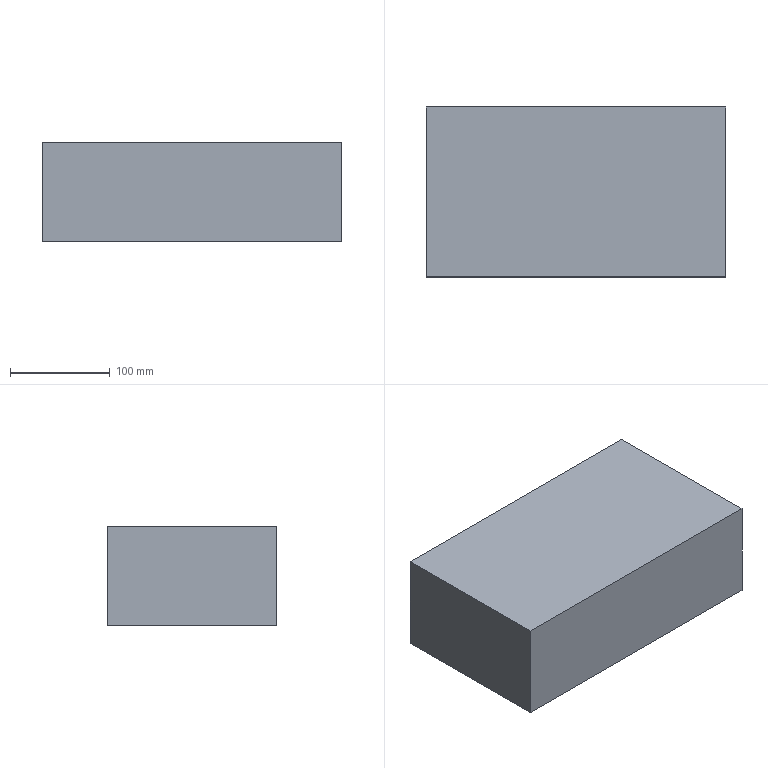Part | SolidWorks | features Extrusion 1 | 1 solid | 6 faces | box 300 x 170 x 100 mm | volume 5100000 mm3 | plane 6
STEP:
#1=CARTESIAN_POINT('',(-150.,85.,50.));
#2=VERTEX_POINT('',#1);
#3=CARTESIAN_POINT('',(-150.,-85.,50.));
#4=VERTEX_POINT('',#3);
#5=CARTESIAN_POINT('',(-150.,85.,50.));
#6=DIRECTION('',(0.,-1.,0.));
#7=VECTOR('',#6,1000.);
#8=LINE('',#5,#7);
#9=EDGE_CURVE('',#2,#4,#8,.T.);
#10=ORIENTED_EDGE('',*,*,#9,.F.);
#11=CARTESIAN_POINT('',(-150.,85.,-50.));
#12=VERTEX_POINT('',#11);
#13=CARTESIAN_POINT('',(-150.,85.,-50.));
#14=DIRECTION('',(0.,0.,1.));
#15=VECTOR('',#14,1000.);
#16=LINE('',#13,#15);
#17=EDGE_CURVE('',#12,#2,#16,.T.);
#18=ORIENTED_EDGE('',*,*,#17,.F.);
#19=CARTESIAN_POINT('',(-150.,-85.,-50.));
#20=VERTEX_POINT('',#19);
#21=CARTESIAN_POINT('',(-150.,85.,-50.));
#22=DIRECTION('',(0.,-1.,0.));
#23=VECTOR('',#22,1000.);
#24=LINE('',#21,#23);
#25=EDGE_CURVE('',#12,#20,#24,.T.);
#26=ORIENTED_EDGE('',*,*,#25,.T.);
#27=CARTESIAN_POINT('',(-150.,-85.,-50.));
#28=DIRECTION('',(0.,0.,1.));
#29=VECTOR('',#28,1000.);
#30=LINE('',#27,#29);
#31=EDGE_CURVE('',#20,#4,#30,.T.);
#32=ORIENTED_EDGE('',*,*,#31,.T.);
#33=EDGE_LOOP('',(#10,#18,#26,#32));
#34=FACE_OUTER_BOUND('',#33,.T.);
#35=CARTESIAN_POINT('',(-150.,85.,-50.));
#36=DIRECTION('',(-1.,0.,0.));
#37=DIRECTION('',(0.,0.,1.));
#38=AXIS2_PLACEMENT_3D('',#35,#36,#37);
#39=PLANE('',#38);
#40=ADVANCED_FACE('',(#34),#39,.T.);
#41=CARTESIAN_POINT('',(150.,85.,50.));
#42=VERTEX_POINT('',#41);
#43=CARTESIAN_POINT('',(150.,85.,50.));
#44=DIRECTION('',(-1.,0.,0.));
#45=VECTOR('',#44,1000.);
#46=LINE('',#43,#45);
#47=EDGE_CURVE('',#42,#2,#46,.T.);
#48=ORIENTED_EDGE('',*,*,#47,.F.);
#49=CARTESIAN_POINT('',(150.,85.,-50.));
#50=VERTEX_POINT('',#49);
#51=CARTESIAN_POINT('',(150.,85.,-50.));
#52=DIRECTION('',(0.,0.,1.));
#53=VECTOR('',#52,1000.);
#54=LINE('',#51,#53);
#55=EDGE_CURVE('',#50,#42,#54,.T.);
#56=ORIENTED_EDGE('',*,*,#55,.F.);
#57=CARTESIAN_POINT('',(150.,85.,-50.));
#58=DIRECTION('',(-1.,0.,0.));
#59=VECTOR('',#58,1000.);
#60=LINE('',#57,#59);
#61=EDGE_CURVE('',#50,#12,#60,.T.);
#62=ORIENTED_EDGE('',*,*,#61,.T.);
#63=ORIENTED_EDGE('',*,*,#17,.T.);
#64=EDGE_LOOP('',(#48,#56,#62,#63));
#65=FACE_OUTER_BOUND('',#64,.T.);
#66=CARTESIAN_POINT('',(150.,85.,-50.));
#67=DIRECTION('',(0.,1.,0.));
#68=DIRECTION('',(0.,0.,1.));
#69=AXIS2_PLACEMENT_3D('',#66,#67,#68);
#70=PLANE('',#69);
#71=ADVANCED_FACE('',(#65),#70,.T.);
#72=CARTESIAN_POINT('',(150.,-85.,50.));
#73=VERTEX_POINT('',#72);
#74=CARTESIAN_POINT('',(150.,-85.,50.));
#75=DIRECTION('',(0.,1.,0.));
#76=VECTOR('',#75,1000.);
#77=LINE('',#74,#76);
#78=EDGE_CURVE('',#73,#42,#77,.T.);
#79=ORIENTED_EDGE('',*,*,#78,.F.);
#80=CARTESIAN_POINT('',(150.,-85.,-50.));
#81=VERTEX_POINT('',#80);
#82=CARTESIAN_POINT('',(150.,-85.,-50.));
#83=DIRECTION('',(0.,0.,1.));
#84=VECTOR('',#83,1000.);
#85=LINE('',#82,#84);
#86=EDGE_CURVE('',#81,#73,#85,.T.);
#87=ORIENTED_EDGE('',*,*,#86,.F.);
#88=CARTESIAN_POINT('',(150.,-85.,-50.));
#89=DIRECTION('',(0.,1.,0.));
#90=VECTOR('',#89,1000.);
#91=LINE('',#88,#90);
#92=EDGE_CURVE('',#81,#50,#91,.T.);
#93=ORIENTED_EDGE('',*,*,#92,.T.);
#94=ORIENTED_EDGE('',*,*,#55,.T.);
#95=EDGE_LOOP('',(#79,#87,#93,#94));
#96=FACE_OUTER_BOUND('',#95,.T.);
#97=CARTESIAN_POINT('',(150.,-85.,-50.));
#98=DIRECTION('',(1.,0.,0.));
#99=DIRECTION('',(0.,0.,-1.));
#100=AXIS2_PLACEMENT_3D('',#97,#98,#99);
#101=PLANE('',#100);
#102=ADVANCED_FACE('',(#96),#101,.T.);
#103=CARTESIAN_POINT('',(-150.,-85.,50.));
#104=DIRECTION('',(1.,0.,0.));
#105=VECTOR('',#104,1000.);
#106=LINE('',#103,#105);
#107=EDGE_CURVE('',#4,#73,#106,.T.);
#108=ORIENTED_EDGE('',*,*,#107,.F.);
#109=ORIENTED_EDGE('',*,*,#31,.F.);
#110=CARTESIAN_POINT('',(-150.,-85.,-50.));
#111=DIRECTION('',(1.,0.,0.));
#112=VECTOR('',#111,1000.);
#113=LINE('',#110,#112);
#114=EDGE_CURVE('',#20,#81,#113,.T.);
#115=ORIENTED_EDGE('',*,*,#114,.T.);
#116=ORIENTED_EDGE('',*,*,#86,.T.);
#117=EDGE_LOOP('',(#108,#109,#115,#116));
#118=FACE_OUTER_BOUND('',#117,.T.);
#119=CARTESIAN_POINT('',(-150.,-85.,-50.));
#120=DIRECTION('',(0.,-1.,0.));
#121=DIRECTION('',(0.,0.,-1.));
#122=AXIS2_PLACEMENT_3D('',#119,#120,#121);
#123=PLANE('',#122);
#124=ADVANCED_FACE('',(#118),#123,.T.);
#125=ORIENTED_EDGE('',*,*,#25,.F.);
#126=ORIENTED_EDGE('',*,*,#61,.F.);
#127=ORIENTED_EDGE('',*,*,#92,.F.);
#128=ORIENTED_EDGE('',*,*,#114,.F.);
#129=EDGE_LOOP('',(#125,#126,#127,#128));
#130=FACE_OUTER_BOUND('',#129,.T.);
#131=CARTESIAN_POINT('',(0.,0.,-50.));
#132=DIRECTION('',(0.,0.,1.));
#133=DIRECTION('',(1.,0.,0.));
#134=AXIS2_PLACEMENT_3D('',#131,#132,#133);
#135=PLANE('',#134);
#136=ADVANCED_FACE('',(#130),#135,.F.);
#137=ORIENTED_EDGE('',*,*,#9,.T.);
#138=ORIENTED_EDGE('',*,*,#107,.T.);
#139=ORIENTED_EDGE('',*,*,#78,.T.);
#140=ORIENTED_EDGE('',*,*,#47,.T.);
#141=EDGE_LOOP('',(#137,#138,#139,#140));
#142=FACE_OUTER_BOUND('',#141,.T.);
#143=CARTESIAN_POINT('',(0.,0.,50.));
#144=DIRECTION('',(0.,0.,1.));
#145=DIRECTION('',(1.,0.,0.));
#146=AXIS2_PLACEMENT_3D('',#143,#144,#145);
#147=PLANE('',#146);
#148=ADVANCED_FACE('',(#142),#147,.T.);
#149=CLOSED_SHELL('',(#40,#71,#102,#124,#136,#148));
#150=MANIFOLD_SOLID_BREP('',#149);
#151=CARTESIAN_POINT('',(0.,0.,0.));
#152=DIRECTION('',(0.,0.,1.));
#153=DIRECTION('',(1.,0.,0.));
#154=AXIS2_PLACEMENT_3D('',#151,#152,#153);
#155=(LENGTH_UNIT()NAMED_UNIT(*)SI_UNIT(.MILLI.,.METRE.));
#156=UNCERTAINTY_MEASURE_WITH_UNIT(LENGTH_MEASURE(0.00001),#155,'','');
#157=(NAMED_UNIT(*)PLANE_ANGLE_UNIT()SI_UNIT($,.RADIAN.));
#158=(NAMED_UNIT(*)SI_UNIT($,.STERADIAN.)SOLID_ANGLE_UNIT());
#159=(GEOMETRIC_REPRESENTATION_CONTEXT(3)GLOBAL_UNCERTAINTY_ASSIGNED_CONTEXT((#156))GLOBAL_UNIT_ASSIGNED_CONTEXT((#155,#157,#158))REPRESENTATION_CONTEXT('',''));
#160=ADVANCED_BREP_SHAPE_REPRESENTATION('',(#150,#154),#159);